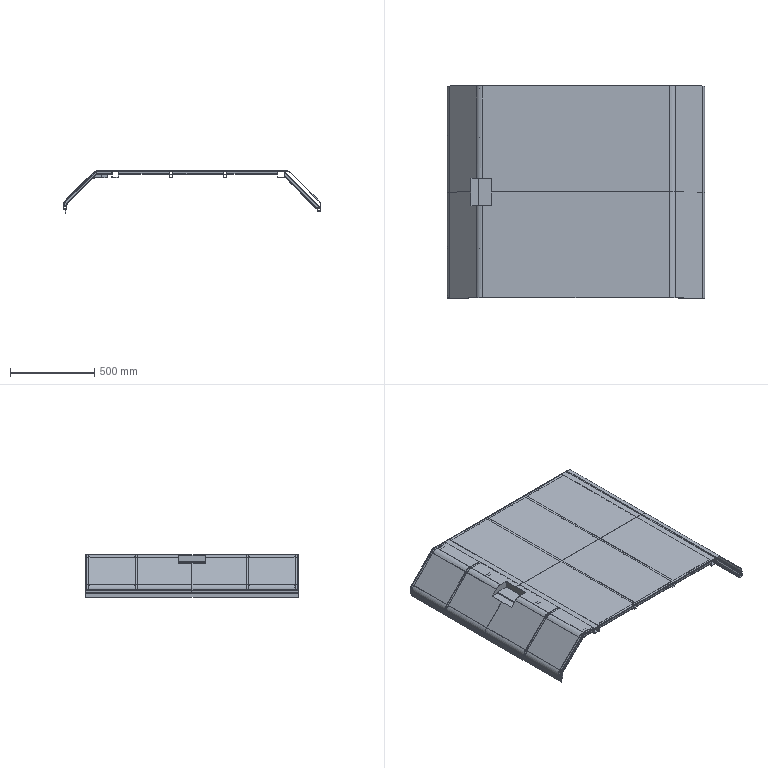Part | NX | features BREP 9 | 34 solids | 1255 faces | box 1528 x 1258 x 253.042 mm | volume 5712882 mm3 | cylinder 617 | plane 557 | torus 64 | spline 17 | commonest cylinder face diameters 6 x120 6.5 x88 4 x74 8 x73 10 x70 7 x56